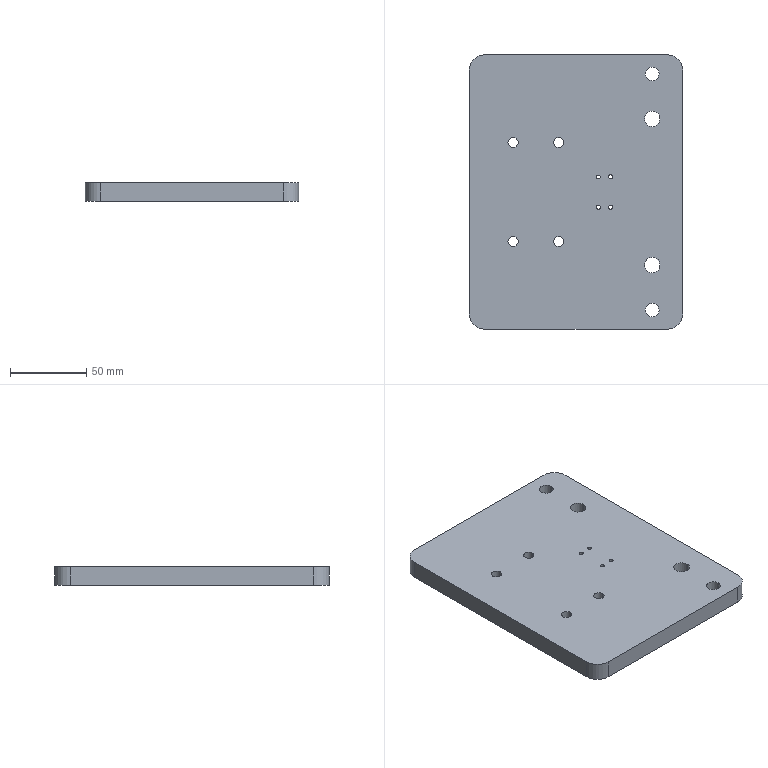Part | STEP file | Base plate 1_Default<Machined> | 1 solid | 34 faces | box 140 x 180 x 12 mm | volume 295903 mm3 | cylinder 28 | plane 6 | commonest cylinder face diameters 2.5 x8 6.8 x8 9 x4 10.2 x4 20 x4
STEP:
#1=CARTESIAN_POINT('',(21.45,-10.,0.));
#2=VERTEX_POINT('',#1);
#3=CARTESIAN_POINT('',(23.95,-10.,0.));
#4=VERTEX_POINT('',#3);
#5=CARTESIAN_POINT('',(22.7,-10.,0.));
#6=DIRECTION('',(0.,0.,1.));
#7=DIRECTION('',(1.,0.,0.));
#8=AXIS2_PLACEMENT_3D('',#5,#6,#7);
#9=CIRCLE('',#8,1.25);
#10=EDGE_CURVE('',#2,#4,#9,.T.);
#11=ORIENTED_EDGE('',*,*,#10,.F.);
#12=CARTESIAN_POINT('',(21.45,-10.,12.));
#13=VERTEX_POINT('',#12);
#14=CARTESIAN_POINT('',(21.45,-10.,12.));
#15=DIRECTION('',(0.,0.,1.));
#16=VECTOR('',#15,1000.);
#17=LINE('',#14,#16);
#18=EDGE_CURVE('',#2,#13,#17,.T.);
#19=ORIENTED_EDGE('',*,*,#18,.T.);
#20=CARTESIAN_POINT('',(23.95,-10.,12.));
#21=VERTEX_POINT('',#20);
#22=CARTESIAN_POINT('',(22.7,-10.,12.));
#23=DIRECTION('',(0.,0.,1.));
#24=DIRECTION('',(1.,0.,0.));
#25=AXIS2_PLACEMENT_3D('',#22,#23,#24);
#26=CIRCLE('',#25,1.25);
#27=EDGE_CURVE('',#13,#21,#26,.T.);
#28=ORIENTED_EDGE('',*,*,#27,.T.);
#29=CARTESIAN_POINT('',(23.95,-10.,12.));
#30=DIRECTION('',(0.,0.,1.));
#31=VECTOR('',#30,1000.);
#32=LINE('',#29,#31);
#33=EDGE_CURVE('',#4,#21,#32,.T.);
#34=ORIENTED_EDGE('',*,*,#33,.F.);
#35=EDGE_LOOP('',(#11,#19,#28,#34));
#36=FACE_OUTER_BOUND('',#35,.T.);
#37=CARTESIAN_POINT('',(22.7,-10.,12.));
#38=DIRECTION('',(0.,0.,1.));
#39=DIRECTION('',(1.,0.,0.));
#40=AXIS2_PLACEMENT_3D('',#37,#38,#39);
#41=CYLINDRICAL_SURFACE('',#40,1.25);
#42=ADVANCED_FACE('',(#36),#41,.F.);
#43=CARTESIAN_POINT('',(13.45,-10.,0.));
#44=VERTEX_POINT('',#43);
#45=CARTESIAN_POINT('',(15.95,-10.,0.));
#46=VERTEX_POINT('',#45);
#47=CARTESIAN_POINT('',(14.7,-10.,0.));
#48=DIRECTION('',(0.,0.,1.));
#49=DIRECTION('',(1.,0.,0.));
#50=AXIS2_PLACEMENT_3D('',#47,#48,#49);
#51=CIRCLE('',#50,1.25);
#52=EDGE_CURVE('',#44,#46,#51,.T.);
#53=ORIENTED_EDGE('',*,*,#52,.F.);
#54=CARTESIAN_POINT('',(13.45,-10.,12.));
#55=VERTEX_POINT('',#54);
#56=CARTESIAN_POINT('',(13.45,-10.,12.));
#57=DIRECTION('',(0.,0.,1.));
#58=VECTOR('',#57,1000.);
#59=LINE('',#56,#58);
#60=EDGE_CURVE('',#44,#55,#59,.T.);
#61=ORIENTED_EDGE('',*,*,#60,.T.);
#62=CARTESIAN_POINT('',(15.95,-10.,12.));
#63=VERTEX_POINT('',#62);
#64=CARTESIAN_POINT('',(14.7,-10.,12.));
#65=DIRECTION('',(0.,0.,1.));
#66=DIRECTION('',(1.,0.,0.));
#67=AXIS2_PLACEMENT_3D('',#64,#65,#66);
#68=CIRCLE('',#67,1.25);
#69=EDGE_CURVE('',#55,#63,#68,.T.);
#70=ORIENTED_EDGE('',*,*,#69,.T.);
#71=CARTESIAN_POINT('',(15.95,-10.,12.));
#72=DIRECTION('',(0.,0.,1.));
#73=VECTOR('',#72,1000.);
#74=LINE('',#71,#73);
#75=EDGE_CURVE('',#46,#63,#74,.T.);
#76=ORIENTED_EDGE('',*,*,#75,.F.);
#77=EDGE_LOOP('',(#53,#61,#70,#76));
#78=FACE_OUTER_BOUND('',#77,.T.);
#79=CARTESIAN_POINT('',(14.7,-10.,12.));
#80=DIRECTION('',(0.,0.,1.));
#81=DIRECTION('',(1.,0.,0.));
#82=AXIS2_PLACEMENT_3D('',#79,#80,#81);
#83=CYLINDRICAL_SURFACE('',#82,1.25);
#84=ADVANCED_FACE('',(#78),#83,.F.);
#85=CARTESIAN_POINT('',(21.45,10.,0.));
#86=VERTEX_POINT('',#85);
#87=CARTESIAN_POINT('',(23.95,10.,0.));
#88=VERTEX_POINT('',#87);
#89=CARTESIAN_POINT('',(22.7,10.,0.));
#90=DIRECTION('',(0.,0.,1.));
#91=DIRECTION('',(1.,0.,0.));
#92=AXIS2_PLACEMENT_3D('',#89,#90,#91);
#93=CIRCLE('',#92,1.25);
#94=EDGE_CURVE('',#86,#88,#93,.T.);
#95=ORIENTED_EDGE('',*,*,#94,.F.);
#96=CARTESIAN_POINT('',(21.45,10.,12.));
#97=VERTEX_POINT('',#96);
#98=CARTESIAN_POINT('',(21.45,10.,12.));
#99=DIRECTION('',(0.,0.,1.));
#100=VECTOR('',#99,1000.);
#101=LINE('',#98,#100);
#102=EDGE_CURVE('',#86,#97,#101,.T.);
#103=ORIENTED_EDGE('',*,*,#102,.T.);
#104=CARTESIAN_POINT('',(23.95,10.,12.));
#105=VERTEX_POINT('',#104);
#106=CARTESIAN_POINT('',(22.7,10.,12.));
#107=DIRECTION('',(0.,0.,1.));
#108=DIRECTION('',(1.,0.,0.));
#109=AXIS2_PLACEMENT_3D('',#106,#107,#108);
#110=CIRCLE('',#109,1.25);
#111=EDGE_CURVE('',#97,#105,#110,.T.);
#112=ORIENTED_EDGE('',*,*,#111,.T.);
#113=CARTESIAN_POINT('',(23.95,10.,12.));
#114=DIRECTION('',(0.,0.,1.));
#115=VECTOR('',#114,1000.);
#116=LINE('',#113,#115);
#117=EDGE_CURVE('',#88,#105,#116,.T.);
#118=ORIENTED_EDGE('',*,*,#117,.F.);
#119=EDGE_LOOP('',(#95,#103,#112,#118));
#120=FACE_OUTER_BOUND('',#119,.T.);
#121=CARTESIAN_POINT('',(22.7,10.,12.));
#122=DIRECTION('',(0.,0.,1.));
#123=DIRECTION('',(1.,0.,0.));
#124=AXIS2_PLACEMENT_3D('',#121,#122,#123);
#125=CYLINDRICAL_SURFACE('',#124,1.25);
#126=ADVANCED_FACE('',(#120),#125,.F.);
#127=CARTESIAN_POINT('',(13.45,9.85,0.));
#128=VERTEX_POINT('',#127);
#129=CARTESIAN_POINT('',(15.95,9.85,0.));
#130=VERTEX_POINT('',#129);
#131=CARTESIAN_POINT('',(14.7,9.85,0.));
#132=DIRECTION('',(0.,0.,1.));
#133=DIRECTION('',(1.,0.,0.));
#134=AXIS2_PLACEMENT_3D('',#131,#132,#133);
#135=CIRCLE('',#134,1.25);
#136=EDGE_CURVE('',#128,#130,#135,.T.);
#137=ORIENTED_EDGE('',*,*,#136,.F.);
#138=CARTESIAN_POINT('',(13.45,9.85,12.));
#139=VERTEX_POINT('',#138);
#140=CARTESIAN_POINT('',(13.45,9.85,12.));
#141=DIRECTION('',(0.,0.,1.));
#142=VECTOR('',#141,1000.);
#143=LINE('',#140,#142);
#144=EDGE_CURVE('',#128,#139,#143,.T.);
#145=ORIENTED_EDGE('',*,*,#144,.T.);
#146=CARTESIAN_POINT('',(15.95,9.85,12.));
#147=VERTEX_POINT('',#146);
#148=CARTESIAN_POINT('',(14.7,9.85,12.));
#149=DIRECTION('',(0.,0.,1.));
#150=DIRECTION('',(1.,0.,0.));
#151=AXIS2_PLACEMENT_3D('',#148,#149,#150);
#152=CIRCLE('',#151,1.25);
#153=EDGE_CURVE('',#139,#147,#152,.T.);
#154=ORIENTED_EDGE('',*,*,#153,.T.);
#155=CARTESIAN_POINT('',(15.95,9.85,12.));
#156=DIRECTION('',(0.,0.,1.));
#157=VECTOR('',#156,1000.);
#158=LINE('',#155,#157);
#159=EDGE_CURVE('',#130,#147,#158,.T.);
#160=ORIENTED_EDGE('',*,*,#159,.F.);
#161=EDGE_LOOP('',(#137,#145,#154,#160));
#162=FACE_OUTER_BOUND('',#161,.T.);
#163=CARTESIAN_POINT('',(14.7,9.85,12.));
#164=DIRECTION('',(0.,0.,1.));
#165=DIRECTION('',(1.,0.,0.));
#166=AXIS2_PLACEMENT_3D('',#163,#164,#165);
#167=CYLINDRICAL_SURFACE('',#166,1.25);
#168=ADVANCED_FACE('',(#162),#167,.F.);
#169=CARTESIAN_POINT('',(45.5,77.5,0.));
#170=VERTEX_POINT('',#169);
#171=CARTESIAN_POINT('',(54.5,77.5,0.));
#172=VERTEX_POINT('',#171);
#173=CARTESIAN_POINT('',(50.,77.5,0.));
#174=DIRECTION('',(0.,0.,1.));
#175=DIRECTION('',(1.,0.,0.));
#176=AXIS2_PLACEMENT_3D('',#173,#174,#175);
#177=CIRCLE('',#176,4.5);
#178=EDGE_CURVE('',#170,#172,#177,.T.);
#179=ORIENTED_EDGE('',*,*,#178,.F.);
#180=CARTESIAN_POINT('',(45.5,77.5,12.));
#181=VERTEX_POINT('',#180);
#182=CARTESIAN_POINT('',(45.5,77.5,12.));
#183=DIRECTION('',(0.,0.,1.));
#184=VECTOR('',#183,1000.);
#185=LINE('',#182,#184);
#186=EDGE_CURVE('',#170,#181,#185,.T.);
#187=ORIENTED_EDGE('',*,*,#186,.T.);
#188=CARTESIAN_POINT('',(54.5,77.5,12.));
#189=VERTEX_POINT('',#188);
#190=CARTESIAN_POINT('',(50.,77.5,12.));
#191=DIRECTION('',(0.,0.,1.));
#192=DIRECTION('',(1.,0.,0.));
#193=AXIS2_PLACEMENT_3D('',#190,#191,#192);
#194=CIRCLE('',#193,4.5);
#195=EDGE_CURVE('',#181,#189,#194,.T.);
#196=ORIENTED_EDGE('',*,*,#195,.T.);
#197=CARTESIAN_POINT('',(54.5,77.5,12.));
#198=DIRECTION('',(0.,0.,1.));
#199=VECTOR('',#198,1000.);
#200=LINE('',#197,#199);
#201=EDGE_CURVE('',#172,#189,#200,.T.);
#202=ORIENTED_EDGE('',*,*,#201,.F.);
#203=EDGE_LOOP('',(#179,#187,#196,#202));
#204=FACE_OUTER_BOUND('',#203,.T.);
#205=CARTESIAN_POINT('',(50.,77.5,12.));
#206=DIRECTION('',(0.,0.,1.));
#207=DIRECTION('',(1.,0.,0.));
#208=AXIS2_PLACEMENT_3D('',#205,#206,#207);
#209=CYLINDRICAL_SURFACE('',#208,4.5);
#210=ADVANCED_FACE('',(#204),#209,.F.);
#211=CARTESIAN_POINT('',(45.5,-77.5,0.));
#212=VERTEX_POINT('',#211);
#213=CARTESIAN_POINT('',(54.5,-77.5,0.));
#214=VERTEX_POINT('',#213);
#215=CARTESIAN_POINT('',(50.,-77.5,0.));
#216=DIRECTION('',(0.,0.,1.));
#217=DIRECTION('',(1.,0.,0.));
#218=AXIS2_PLACEMENT_3D('',#215,#216,#217);
#219=CIRCLE('',#218,4.5);
#220=EDGE_CURVE('',#212,#214,#219,.T.);
#221=ORIENTED_EDGE('',*,*,#220,.F.);
#222=CARTESIAN_POINT('',(45.5,-77.5,12.));
#223=VERTEX_POINT('',#222);
#224=CARTESIAN_POINT('',(45.5,-77.5,12.));
#225=DIRECTION('',(0.,0.,1.));
#226=VECTOR('',#225,1000.);
#227=LINE('',#224,#226);
#228=EDGE_CURVE('',#212,#223,#227,.T.);
#229=ORIENTED_EDGE('',*,*,#228,.T.);
#230=CARTESIAN_POINT('',(54.5,-77.5,12.));
#231=VERTEX_POINT('',#230);
#232=CARTESIAN_POINT('',(50.,-77.5,12.));
#233=DIRECTION('',(0.,0.,1.));
#234=DIRECTION('',(1.,0.,0.));
#235=AXIS2_PLACEMENT_3D('',#232,#233,#234);
#236=CIRCLE('',#235,4.5);
#237=EDGE_CURVE('',#223,#231,#236,.T.);
#238=ORIENTED_EDGE('',*,*,#237,.T.);
#239=CARTESIAN_POINT('',(54.5,-77.5,12.));
#240=DIRECTION('',(0.,0.,1.));
#241=VECTOR('',#240,1000.);
#242=LINE('',#239,#241);
#243=EDGE_CURVE('',#214,#231,#242,.T.);
#244=ORIENTED_EDGE('',*,*,#243,.F.);
#245=EDGE_LOOP('',(#221,#229,#238,#244));
#246=FACE_OUTER_BOUND('',#245,.T.);
#247=CARTESIAN_POINT('',(50.,-77.5,12.));
#248=DIRECTION('',(0.,0.,1.));
#249=DIRECTION('',(1.,0.,0.));
#250=AXIS2_PLACEMENT_3D('',#247,#248,#249);
#251=CYLINDRICAL_SURFACE('',#250,4.5);
#252=ADVANCED_FACE('',(#246),#251,.F.);
#253=CARTESIAN_POINT('',(44.9,48.,0.));
#254=VERTEX_POINT('',#253);
#255=CARTESIAN_POINT('',(55.1,48.,0.));
#256=VERTEX_POINT('',#255);
#257=CARTESIAN_POINT('',(50.,48.,0.));
#258=DIRECTION('',(0.,0.,1.));
#259=DIRECTION('',(1.,0.,0.));
#260=AXIS2_PLACEMENT_3D('',#257,#258,#259);
#261=CIRCLE('',#260,5.1);
#262=EDGE_CURVE('',#254,#256,#261,.T.);
#263=ORIENTED_EDGE('',*,*,#262,.F.);
#264=CARTESIAN_POINT('',(44.9,48.,12.));
#265=VERTEX_POINT('',#264);
#266=CARTESIAN_POINT('',(44.9,48.,12.));
#267=DIRECTION('',(0.,0.,1.));
#268=VECTOR('',#267,1000.);
#269=LINE('',#266,#268);
#270=EDGE_CURVE('',#254,#265,#269,.T.);
#271=ORIENTED_EDGE('',*,*,#270,.T.);
#272=CARTESIAN_POINT('',(55.1,48.,12.));
#273=VERTEX_POINT('',#272);
#274=CARTESIAN_POINT('',(50.,48.,12.));
#275=DIRECTION('',(0.,0.,1.));
#276=DIRECTION('',(1.,0.,0.));
#277=AXIS2_PLACEMENT_3D('',#274,#275,#276);
#278=CIRCLE('',#277,5.1);
#279=EDGE_CURVE('',#265,#273,#278,.T.);
#280=ORIENTED_EDGE('',*,*,#279,.T.);
#281=CARTESIAN_POINT('',(55.1,48.,12.));
#282=DIRECTION('',(0.,0.,1.));
#283=VECTOR('',#282,1000.);
#284=LINE('',#281,#283);
#285=EDGE_CURVE('',#256,#273,#284,.T.);
#286=ORIENTED_EDGE('',*,*,#285,.F.);
#287=EDGE_LOOP('',(#263,#271,#280,#286));
#288=FACE_OUTER_BOUND('',#287,.T.);
#289=CARTESIAN_POINT('',(50.,48.,12.));
#290=DIRECTION('',(0.,0.,1.));
#291=DIRECTION('',(1.,0.,0.));
#292=AXIS2_PLACEMENT_3D('',#289,#290,#291);
#293=CYLINDRICAL_SURFACE('',#292,5.1);
#294=ADVANCED_FACE('',(#288),#293,.F.);
#295=CARTESIAN_POINT('',(44.9,-48.,0.));
#296=VERTEX_POINT('',#295);
#297=CARTESIAN_POINT('',(55.1,-48.,0.));
#298=VERTEX_POINT('',#297);
#299=CARTESIAN_POINT('',(50.,-48.,0.));
#300=DIRECTION('',(0.,0.,1.));
#301=DIRECTION('',(1.,0.,0.));
#302=AXIS2_PLACEMENT_3D('',#299,#300,#301);
#303=CIRCLE('',#302,5.1);
#304=EDGE_CURVE('',#296,#298,#303,.T.);
#305=ORIENTED_EDGE('',*,*,#304,.F.);
#306=CARTESIAN_POINT('',(44.9,-48.,12.));
#307=VERTEX_POINT('',#306);
#308=CARTESIAN_POINT('',(44.9,-48.,12.));
#309=DIRECTION('',(0.,0.,1.));
#310=VECTOR('',#309,1000.);
#311=LINE('',#308,#310);
#312=EDGE_CURVE('',#296,#307,#311,.T.);
#313=ORIENTED_EDGE('',*,*,#312,.T.);
#314=CARTESIAN_POINT('',(55.1,-48.,12.));
#315=VERTEX_POINT('',#314);
#316=CARTESIAN_POINT('',(50.,-48.,12.));
#317=DIRECTION('',(0.,0.,1.));
#318=DIRECTION('',(1.,0.,0.));
#319=AXIS2_PLACEMENT_3D('',#316,#317,#318);
#320=CIRCLE('',#319,5.1);
#321=EDGE_CURVE('',#307,#315,#320,.T.);
#322=ORIENTED_EDGE('',*,*,#321,.T.);
#323=CARTESIAN_POINT('',(55.1,-48.,12.));
#324=DIRECTION('',(0.,0.,1.));
#325=VECTOR('',#324,1000.);
#326=LINE('',#323,#325);
#327=EDGE_CURVE('',#298,#315,#326,.T.);
#328=ORIENTED_EDGE('',*,*,#327,.F.);
#329=EDGE_LOOP('',(#305,#313,#322,#328));
#330=FACE_OUTER_BOUND('',#329,.T.);
#331=CARTESIAN_POINT('',(50.,-48.,12.));
#332=DIRECTION('',(0.,0.,1.));
#333=DIRECTION('',(1.,0.,0.));
#334=AXIS2_PLACEMENT_3D('',#331,#332,#333);
#335=CYLINDRICAL_SURFACE('',#334,5.1);
#336=ADVANCED_FACE('',(#330),#335,.F.);
#337=CARTESIAN_POINT('',(-14.7,32.5,0.));
#338=VERTEX_POINT('',#337);
#339=CARTESIAN_POINT('',(-7.9,32.5,0.));
#340=VERTEX_POINT('',#339);
#341=CARTESIAN_POINT('',(-11.3,32.5,0.));
#342=DIRECTION('',(0.,0.,1.));
#343=DIRECTION('',(1.,0.,0.));
#344=AXIS2_PLACEMENT_3D('',#341,#342,#343);
#345=CIRCLE('',#344,3.4);
#346=EDGE_CURVE('',#338,#340,#345,.T.);
#347=ORIENTED_EDGE('',*,*,#346,.F.);
#348=CARTESIAN_POINT('',(-14.7,32.5,12.));
#349=VERTEX_POINT('',#348);
#350=CARTESIAN_POINT('',(-14.7,32.5,12.));
#351=DIRECTION('',(0.,0.,1.));
#352=VECTOR('',#351,1000.);
#353=LINE('',#350,#352);
#354=EDGE_CURVE('',#338,#349,#353,.T.);
#355=ORIENTED_EDGE('',*,*,#354,.T.);
#356=CARTESIAN_POINT('',(-7.9,32.5,12.));
#357=VERTEX_POINT('',#356);
#358=CARTESIAN_POINT('',(-11.3,32.5,12.));
#359=DIRECTION('',(0.,0.,1.));
#360=DIRECTION('',(1.,0.,0.));
#361=AXIS2_PLACEMENT_3D('',#358,#359,#360);
#362=CIRCLE('',#361,3.4);
#363=EDGE_CURVE('',#349,#357,#362,.T.);
#364=ORIENTED_EDGE('',*,*,#363,.T.);
#365=CARTESIAN_POINT('',(-7.9,32.5,12.));
#366=DIRECTION('',(0.,0.,1.));
#367=VECTOR('',#366,1000.);
#368=LINE('',#365,#367);
#369=EDGE_CURVE('',#340,#357,#368,.T.);
#370=ORIENTED_EDGE('',*,*,#369,.F.);
#371=EDGE_LOOP('',(#347,#355,#364,#370));
#372=FACE_OUTER_BOUND('',#371,.T.);
#373=CARTESIAN_POINT('',(-11.3,32.5,12.));
#374=DIRECTION('',(0.,0.,1.));
#375=DIRECTION('',(1.,0.,0.));
#376=AXIS2_PLACEMENT_3D('',#373,#374,#375);
#377=CYLINDRICAL_SURFACE('',#376,3.4);
#378=ADVANCED_FACE('',(#372),#377,.F.);
#379=CARTESIAN_POINT('',(-44.7,32.5,0.));
#380=VERTEX_POINT('',#379);
#381=CARTESIAN_POINT('',(-37.9,32.5,0.));
#382=VERTEX_POINT('',#381);
#383=CARTESIAN_POINT('',(-41.3,32.5,0.));
#384=DIRECTION('',(0.,0.,1.));
#385=DIRECTION('',(1.,0.,0.));
#386=AXIS2_PLACEMENT_3D('',#383,#384,#385);
#387=CIRCLE('',#386,3.4);
#388=EDGE_CURVE('',#380,#382,#387,.T.);
#389=ORIENTED_EDGE('',*,*,#388,.F.);
#390=CARTESIAN_POINT('',(-44.7,32.5,12.));
#391=VERTEX_POINT('',#390);
#392=CARTESIAN_POINT('',(-44.7,32.5,12.));
#393=DIRECTION('',(0.,0.,1.));
#394=VECTOR('',#393,1000.);
#395=LINE('',#392,#394);
#396=EDGE_CURVE('',#380,#391,#395,.T.);
#397=ORIENTED_EDGE('',*,*,#396,.T.);
#398=CARTESIAN_POINT('',(-37.9,32.5,12.));
#399=VERTEX_POINT('',#398);
#400=CARTESIAN_POINT('',(-41.3,32.5,12.));
#401=DIRECTION('',(0.,0.,1.));
#402=DIRECTION('',(1.,0.,0.));
#403=AXIS2_PLACEMENT_3D('',#400,#401,#402);
#404=CIRCLE('',#403,3.4);
#405=EDGE_CURVE('',#391,#399,#404,.T.);
#406=ORIENTED_EDGE('',*,*,#405,.T.);
#407=CARTESIAN_POINT('',(-37.9,32.5,12.));
#408=DIRECTION('',(0.,0.,1.));
#409=VECTOR('',#408,1000.);
#410=LINE('',#407,#409);
#411=EDGE_CURVE('',#382,#399,#410,.T.);
#412=ORIENTED_EDGE('',*,*,#411,.F.);
#413=EDGE_LOOP('',(#389,#397,#406,#412));
#414=FACE_OUTER_BOUND('',#413,.T.);
#415=CARTESIAN_POINT('',(-41.3,32.5,12.));
#416=DIRECTION('',(0.,0.,1.));
#417=DIRECTION('',(1.,0.,0.));
#418=AXIS2_PLACEMENT_3D('',#415,#416,#417);
#419=CYLINDRICAL_SURFACE('',#418,3.4);
#420=ADVANCED_FACE('',(#414),#419,.F.);
#421=CARTESIAN_POINT('',(-14.7,-32.5,0.));
#422=VERTEX_POINT('',#421);
#423=CARTESIAN_POINT('',(-7.9,-32.5,0.));
#424=VERTEX_POINT('',#423);
#425=CARTESIAN_POINT('',(-11.3,-32.5,0.));
#426=DIRECTION('',(0.,0.,1.));
#427=DIRECTION('',(1.,0.,0.));
#428=AXIS2_PLACEMENT_3D('',#425,#426,#427);
#429=CIRCLE('',#428,3.4);
#430=EDGE_CURVE('',#422,#424,#429,.T.);
#431=ORIENTED_EDGE('',*,*,#430,.F.);
#432=CARTESIAN_POINT('',(-14.7,-32.5,12.));
#433=VERTEX_POINT('',#432);
#434=CARTESIAN_POINT('',(-14.7,-32.5,12.));
#435=DIRECTION('',(0.,0.,1.));
#436=VECTOR('',#435,1000.);
#437=LINE('',#434,#436);
#438=EDGE_CURVE('',#422,#433,#437,.T.);
#439=ORIENTED_EDGE('',*,*,#438,.T.);
#440=CARTESIAN_POINT('',(-7.9,-32.5,12.));
#441=VERTEX_POINT('',#440);
#442=CARTESIAN_POINT('',(-11.3,-32.5,12.));
#443=DIRECTION('',(0.,0.,1.));
#444=DIRECTION('',(1.,0.,0.));
#445=AXIS2_PLACEMENT_3D('',#442,#443,#444);
#446=CIRCLE('',#445,3.4);
#447=EDGE_CURVE('',#433,#441,#446,.T.);
#448=ORIENTED_EDGE('',*,*,#447,.T.);
#449=CARTESIAN_POINT('',(-7.9,-32.5,12.));
#450=DIRECTION('',(0.,0.,1.));
#451=VECTOR('',#450,1000.);
#452=LINE('',#449,#451);
#453=EDGE_CURVE('',#424,#441,#452,.T.);
#454=ORIENTED_EDGE('',*,*,#453,.F.);
#455=EDGE_LOOP('',(#431,#439,#448,#454));
#456=FACE_OUTER_BOUND('',#455,.T.);
#457=CARTESIAN_POINT('',(-11.3,-32.5,12.));
#458=DIRECTION('',(0.,0.,1.));
#459=DIRECTION('',(1.,0.,0.));
#460=AXIS2_PLACEMENT_3D('',#457,#458,#459);
#461=CYLINDRICAL_SURFACE('',#460,3.4);
#462=ADVANCED_FACE('',(#456),#461,.F.);
#463=CARTESIAN_POINT('',(-44.7,-32.5,0.));
#464=VERTEX_POINT('',#463);
#465=CARTESIAN_POINT('',(-37.9,-32.5,0.));
#466=VERTEX_POINT('',#465);
#467=CARTESIAN_POINT('',(-41.3,-32.5,0.));
#468=DIRECTION('',(0.,0.,1.));
#469=DIRECTION('',(1.,0.,0.));
#470=AXIS2_PLACEMENT_3D('',#467,#468,#469);
#471=CIRCLE('',#470,3.4);
#472=EDGE_CURVE('',#464,#466,#471,.T.);
#473=ORIENTED_EDGE('',*,*,#472,.F.);
#474=CARTESIAN_POINT('',(-44.7,-32.5,12.));
#475=VERTEX_POINT('',#474);
#476=CARTESIAN_POINT('',(-44.7,-32.5,12.));
#477=DIRECTION('',(0.,0.,1.));
#478=VECTOR('',#477,1000.);
#479=LINE('',#476,#478);
#480=EDGE_CURVE('',#464,#475,#479,.T.);
#481=ORIENTED_EDGE('',*,*,#480,.T.);
#482=CARTESIAN_POINT('',(-37.9,-32.5,12.));
#483=VERTEX_POINT('',#482);
#484=CARTESIAN_POINT('',(-41.3,-32.5,12.));
#485=DIRECTION('',(0.,0.,1.));
#486=DIRECTION('',(1.,0.,0.));
#487=AXIS2_PLACEMENT_3D('',#484,#485,#486);
#488=CIRCLE('',#487,3.4);
#489=EDGE_CURVE('',#475,#483,#488,.T.);
#490=ORIENTED_EDGE('',*,*,#489,.T.);
#491=CARTESIAN_POINT('',(-37.9,-32.5,12.));
#492=DIRECTION('',(0.,0.,1.));
#493=VECTOR('',#492,1000.);
#494=LINE('',#491,#493);
#495=EDGE_CURVE('',#466,#483,#494,.T.);
#496=ORIENTED_EDGE('',*,*,#495,.F.);
#497=EDGE_LOOP('',(#473,#481,#490,#496));
#498=FACE_OUTER_BOUND('',#497,.T.);
#499=CARTESIAN_POINT('',(-41.3,-32.5,12.));
#500=DIRECTION('',(0.,0.,1.));
#501=DIRECTION('',(1.,0.,0.));
#502=AXIS2_PLACEMENT_3D('',#499,#500,#501);
#503=CYLINDRICAL_SURFACE('',#502,3.4);
#504=ADVANCED_FACE('',(#498),#503,.F.);
#505=CARTESIAN_POINT('',(70.,-80.,12.));
#506=VERTEX_POINT('',#505);
#507=CARTESIAN_POINT('',(70.,80.,12.));
#508=VERTEX_POINT('',#507);
#509=CARTESIAN_POINT('',(70.,90.,12.));
#510=DIRECTION('',(0.,1.,0.));
#511=VECTOR('',#510,1000.);
#512=LINE('',#509,#511);
#513=EDGE_CURVE('',#506,#508,#512,.T.);
#514=ORIENTED_EDGE('',*,*,#513,.F.);
#515=CARTESIAN_POINT('',(70.,-80.,0.));
#516=VERTEX_POINT('',#515);
#517=CARTESIAN_POINT('',(70.,-80.,12.));
#518=DIRECTION('',(0.,0.,-1.));
#519=VECTOR('',#518,1000.);
#520=LINE('',#517,#519);
#521=EDGE_CURVE('',#506,#516,#520,.T.);
#522=ORIENTED_EDGE('',*,*,#521,.T.);
#523=CARTESIAN_POINT('',(70.,80.,0.));
#524=VERTEX_POINT('',#523);
#525=CARTESIAN_POINT('',(70.,90.,0.));
#526=DIRECTION('',(0.,1.,0.));
#527=VECTOR('',#526,1000.);
#528=LINE('',#525,#527);
#529=EDGE_CURVE('',#516,#524,#528,.T.);
#530=ORIENTED_EDGE('',*,*,#529,.T.);
#531=CARTESIAN_POINT('',(70.,80.,12.));
#532=DIRECTION('',(0.,0.,1.));
#533=VECTOR('',#532,1000.);
#534=LINE('',#531,#533);
#535=EDGE_CURVE('',#524,#508,#534,.T.);
#536=ORIENTED_EDGE('',*,*,#535,.T.);
#537=EDGE_LOOP('',(#514,#522,#530,#536));
#538=FACE_OUTER_BOUND('',#537,.T.);
#539=CARTESIAN_POINT('',(70.,90.,12.));
#540=DIRECTION('',(-1.,0.,0.));
#541=DIRECTION('',(0.,-1.,0.));
#542=AXIS2_PLACEMENT_3D('',#539,#540,#541);
#543=PLANE('',#542);
#544=ADVANCED_FACE('',(#538),#543,.F.);
#545=CARTESIAN_POINT('',(60.,90.,12.));
#546=VERTEX_POINT('',#545);
#547=CARTESIAN_POINT('',(-60.,90.,12.));
#548=VERTEX_POINT('',#547);
#549=CARTESIAN_POINT('',(-70.,90.,12.));
#550=DIRECTION('',(-1.,0.,0.));
#551=VECTOR('',#550,1000.);
#552=LINE('',#549,#551);
#553=EDGE_CURVE('',#546,#548,#552,.T.);
#554=ORIENTED_EDGE('',*,*,#553,.F.);
#555=CARTESIAN_POINT('',(60.,90.,0.));
#556=VERTEX_POINT('',#555);
#557=CARTESIAN_POINT('',(60.,90.,12.));
#558=DIRECTION('',(0.,0.,-1.));
#559=VECTOR('',#558,1000.);
#560=LINE('',#557,#559);
#561=EDGE_CURVE('',#546,#556,#560,.T.);
#562=ORIENTED_EDGE('',*,*,#561,.T.);
#563=CARTESIAN_POINT('',(-60.,90.,0.));
#564=VERTEX_POINT('',#563);
#565=CARTESIAN_POINT('',(-70.,90.,0.));
#566=DIRECTION('',(-1.,0.,0.));
#567=VECTOR('',#566,1000.);
#568=LINE('',#565,#567);
#569=EDGE_CURVE('',#556,#564,#568,.T.);
#570=ORIENTED_EDGE('',*,*,#569,.T.);
#571=CARTESIAN_POINT('',(-60.,90.,12.));
#572=DIRECTION('',(0.,0.,1.));
#573=VECTOR('',#572,1000.);
#574=LINE('',#571,#573);
#575=EDGE_CURVE('',#564,#548,#574,.T.);
#576=ORIENTED_EDGE('',*,*,#575,.T.);
#577=EDGE_LOOP('',(#554,#562,#570,#576));
#578=FACE_OUTER_BOUND('',#577,.T.);
#579=CARTESIAN_POINT('',(-70.,90.,12.));
#580=DIRECTION('',(0.,-1.,0.));
#581=DIRECTION('',(0.,0.,-1.));
#582=AXIS2_PLACEMENT_3D('',#579,#580,#581);
#583=PLANE('',#582);
#584=ADVANCED_FACE('',(#578),#583,.F.);
#585=CARTESIAN_POINT('',(-70.,80.,0.));
#586=VERTEX_POINT('',#585);
#587=CARTESIAN_POINT('',(-70.,-80.,0.));
#588=VERTEX_POINT('',#587);
#589=CARTESIAN_POINT('',(-70.,90.,0.));
#590=DIRECTION('',(0.,-1.,0.));
#591=VECTOR('',#590,1000.);
#592=LINE('',#589,#591);
#593=EDGE_CURVE('',#586,#588,#592,.T.);
#594=ORIENTED_EDGE('',*,*,#593,.T.);
#595=CARTESIAN_POINT('',(-70.,-80.,12.));
#596=VERTEX_POINT('',#595);
#597=CARTESIAN_POINT('',(-70.,-80.,12.));
#598=DIRECTION('',(0.,0.,1.));
#599=VECTOR('',#598,1000.);
#600=LINE('',#597,#599);
#601=EDGE_CURVE('',#588,#596,#600,.T.);
#602=ORIENTED_EDGE('',*,*,#601,.T.);
#603=CARTESIAN_POINT('',(-70.,80.,12.));
#604=VERTEX_POINT('',#603);
#605=CARTESIAN_POINT('',(-70.,90.,12.));
#606=DIRECTION('',(0.,-1.,0.));
#607=VECTOR('',#606,1000.);
#608=LINE('',#605,#607);
#609=EDGE_CURVE('',#604,#596,#608,.T.);
#610=ORIENTED_EDGE('',*,*,#609,.F.);
#611=CARTESIAN_POINT('',(-70.,80.,12.));
#612=DIRECTION('',(0.,0.,-1.));
#613=VECTOR('',#612,1000.);
#614=LINE('',#611,#613);
#615=EDGE_CURVE('',#604,#586,#614,.T.);
#616=ORIENTED_EDGE('',*,*,#615,.T.);
#617=EDGE_LOOP('',(#594,#602,#610,#616));
#618=FACE_OUTER_BOUND('',#617,.T.);
#619=CARTESIAN_POINT('',(-70.,90.,12.));
#620=DIRECTION('',(1.,0.,0.));
#621=DIRECTION('',(0.,1.,0.));
#622=AXIS2_PLACEMENT_3D('',#619,#620,#621);
#623=PLANE('',#622);
#624=ADVANCED_FACE('',(#618),#623,.F.);
#625=CARTESIAN_POINT('',(-60.,-90.,12.));
#626=VERTEX_POINT('',#625);
#627=CARTESIAN_POINT('',(60.,-90.,12.));
#628=VERTEX_POINT('',#627);
#629=CARTESIAN_POINT('',(-70.,-90.,12.));
#630=DIRECTION('',(1.,0.,0.));
#631=VECTOR('',#630,1000.);
#632=LINE('',#629,#631);
#633=EDGE_CURVE('',#626,#628,#632,.T.);
#634=ORIENTED_EDGE('',*,*,#633,.F.);
#635=CARTESIAN_POINT('',(-60.,-90.,0.));
#636=VERTEX_POINT('',#635);
#637=CARTESIAN_POINT('',(-60.,-90.,12.));
#638=DIRECTION('',(0.,0.,-1.));
#639=VECTOR('',#638,1000.);
#640=LINE('',#637,#639);
#641=EDGE_CURVE('',#626,#636,#640,.T.);
#642=ORIENTED_EDGE('',*,*,#641,.T.);
#643=CARTESIAN_POINT('',(60.,-90.,0.));
#644=VERTEX_POINT('',#643);
#645=CARTESIAN_POINT('',(-70.,-90.,0.));
#646=DIRECTION('',(1.,0.,0.));
#647=VECTOR('',#646,1000.);
#648=LINE('',#645,#647);
#649=EDGE_CURVE('',#636,#644,#648,.T.);
#650=ORIENTED_EDGE('',*,*,#649,.T.);
#651=CARTESIAN_POINT('',(60.,-90.,12.));
#652=DIRECTION('',(0.,0.,1.));
#653=VECTOR('',#652,1000.);
#654=LINE('',#651,#653);
#655=EDGE_CURVE('',#644,#628,#654,.T.);
#656=ORIENTED_EDGE('',*,*,#655,.T.);
#657=EDGE_LOOP('',(#634,#642,#650,#656));
#658=FACE_OUTER_BOUND('',#657,.T.);
#659=CARTESIAN_POINT('',(-70.,-90.,12.));
#660=DIRECTION('',(0.,1.,0.));
#661=DIRECTION('',(0.,0.,1.));
#662=AXIS2_PLACEMENT_3D('',#659,#660,#661);
#663=PLANE('',#662);
#664=ADVANCED_FACE('',(#658),#663,.F.);
#665=CARTESIAN_POINT('',(22.7,-10.,12.));
#666=DIRECTION('',(0.,0.,1.));
#667=DIRECTION('',(1.,0.,0.));
#668=AXIS2_PLACEMENT_3D('',#665,#666,#667);
#669=CIRCLE('',#668,1.25);
#670=EDGE_CURVE('',#21,#13,#669,.T.);
#671=ORIENTED_EDGE('',*,*,#670,.F.);
#672=ORIENTED_EDGE('',*,*,#27,.F.);
#673=EDGE_LOOP('',(#671,#672));
#674=FACE_BOUND('',#673,.T.);
#675=CARTESIAN_POINT('',(14.7,-10.,12.));
#676=DIRECTION('',(0.,0.,1.));
#677=DIRECTION('',(1.,0.,0.));
#678=AXIS2_PLACEMENT_3D('',#675,#676,#677);
#679=CIRCLE('',#678,1.25);
#680=EDGE_CURVE('',#63,#55,#679,.T.);
#681=ORIENTED_EDGE('',*,*,#680,.F.);
#682=ORIENTED_EDGE('',*,*,#69,.F.);
#683=EDGE_LOOP('',(#681,#682));
#684=FACE_BOUND('',#683,.T.);
#685=CARTESIAN_POINT('',(22.7,10.,12.));
#686=DIRECTION('',(0.,0.,1.));
#687=DIRECTION('',(1.,0.,0.));
#688=AXIS2_PLACEMENT_3D('',#685,#686,#687);
#689=CIRCLE('',#688,1.25);
#690=EDGE_CURVE('',#105,#97,#689,.T.);
#691=ORIENTED_EDGE('',*,*,#690,.F.);
#692=ORIENTED_EDGE('',*,*,#111,.F.);
#693=EDGE_LOOP('',(#691,#692));
#694=FACE_BOUND('',#693,.T.);
#695=CARTESIAN_POINT('',(14.7,9.85,12.));
#696=DIRECTION('',(0.,0.,1.));
#697=DIRECTION('',(1.,0.,0.));
#698=AXIS2_PLACEMENT_3D('',#695,#696,#697);
#699=CIRCLE('',#698,1.25);
#700=EDGE_CURVE('',#147,#139,#699,.T.);
#701=ORIENTED_EDGE('',*,*,#700,.F.);
#702=ORIENTED_EDGE('',*,*,#153,.F.);
#703=EDGE_LOOP('',(#701,#702));
#704=FACE_BOUND('',#703,.T.);
#705=CARTESIAN_POINT('',(50.,77.5,12.));
#706=DIRECTION('',(0.,0.,1.));
#707=DIRECTION('',(1.,0.,0.));
#708=AXIS2_PLACEMENT_3D('',#705,#706,#707);
#709=CIRCLE('',#708,4.5);
#710=EDGE_CURVE('',#189,#181,#709,.T.);
#711=ORIENTED_EDGE('',*,*,#710,.F.);
#712=ORIENTED_EDGE('',*,*,#195,.F.);
#713=EDGE_LOOP('',(#711,#712));
#714=FACE_BOUND('',#713,.T.);
#715=CARTESIAN_POINT('',(50.,-77.5,12.));
#716=DIRECTION('',(0.,0.,1.));
#717=DIRECTION('',(1.,0.,0.));
#718=AXIS2_PLACEMENT_3D('',#715,#716,#717);
#719=CIRCLE('',#718,4.5);
#720=EDGE_CURVE('',#231,#223,#719,.T.);
#721=ORIENTED_EDGE('',*,*,#720,.F.);
#722=ORIENTED_EDGE('',*,*,#237,.F.);
#723=EDGE_LOOP('',(#721,#722));
#724=FACE_BOUND('',#723,.T.);
#725=CARTESIAN_POINT('',(50.,48.,12.));
#726=DIRECTION('',(0.,0.,1.));
#727=DIRECTION('',(1.,0.,0.));
#728=AXIS2_PLACEMENT_3D('',#725,#726,#727);
#729=CIRCLE('',#728,5.1);
#730=EDGE_CURVE('',#273,#265,#729,.T.);
#731=ORIENTED_EDGE('',*,*,#730,.F.);
#732=ORIENTED_EDGE('',*,*,#279,.F.);
#733=EDGE_LOOP('',(#731,#732));
#734=FACE_BOUND('',#733,.T.);
#735=CARTESIAN_POINT('',(50.,-48.,12.));
#736=DIRECTION('',(0.,0.,1.));
#737=DIRECTION('',(1.,0.,0.));
#738=AXIS2_PLACEMENT_3D('',#735,#736,#737);
#739=CIRCLE('',#738,5.1);
#740=EDGE_CURVE('',#315,#307,#739,.T.);
#741=ORIENTED_EDGE('',*,*,#740,.F.);
#742=ORIENTED_EDGE('',*,*,#321,.F.);
#743=EDGE_LOOP('',(#741,#742));
#744=FACE_BOUND('',#743,.T.);
#745=CARTESIAN_POINT('',(-11.3,32.5,12.));
#746=DIRECTION('',(0.,0.,1.));
#747=DIRECTION('',(1.,0.,0.));
#748=AXIS2_PLACEMENT_3D('',#745,#746,#747);
#749=CIRCLE('',#748,3.4);
#750=EDGE_CURVE('',#357,#349,#749,.T.);
#751=ORIENTED_EDGE('',*,*,#750,.F.);
#752=ORIENTED_EDGE('',*,*,#363,.F.);
#753=EDGE_LOOP('',(#751,#752));
#754=FACE_BOUND('',#753,.T.);
#755=CARTESIAN_POINT('',(-41.3,32.5,12.));
#756=DIRECTION('',(0.,0.,1.));
#757=DIRECTION('',(1.,0.,0.));
#758=AXIS2_PLACEMENT_3D('',#755,#756,#757);
#759=CIRCLE('',#758,3.4);
#760=EDGE_CURVE('',#399,#391,#759,.T.);
#761=ORIENTED_EDGE('',*,*,#760,.F.);
#762=ORIENTED_EDGE('',*,*,#405,.F.);
#763=EDGE_LOOP('',(#761,#762));
#764=FACE_BOUND('',#763,.T.);
#765=CARTESIAN_POINT('',(-11.3,-32.5,12.));
#766=DIRECTION('',(0.,0.,1.));
#767=DIRECTION('',(1.,0.,0.));
#768=AXIS2_PLACEMENT_3D('',#765,#766,#767);
#769=CIRCLE('',#768,3.4);
#770=EDGE_CURVE('',#441,#433,#769,.T.);
#771=ORIENTED_EDGE('',*,*,#770,.F.);
#772=ORIENTED_EDGE('',*,*,#447,.F.);
#773=EDGE_LOOP('',(#771,#772));
#774=FACE_BOUND('',#773,.T.);
#775=CARTESIAN_POINT('',(-41.3,-32.5,12.));
#776=DIRECTION('',(0.,0.,1.));
#777=DIRECTION('',(1.,0.,0.));
#778=AXIS2_PLACEMENT_3D('',#775,#776,#777);
#779=CIRCLE('',#778,3.4);
#780=EDGE_CURVE('',#483,#475,#779,.T.);
#781=ORIENTED_EDGE('',*,*,#780,.F.);
#782=ORIENTED_EDGE('',*,*,#489,.F.);
#783=EDGE_LOOP('',(#781,#782));
#784=FACE_BOUND('',#783,.T.);
#785=ORIENTED_EDGE('',*,*,#609,.T.);
#786=CARTESIAN_POINT('',(-60.,-80.,12.));
#787=DIRECTION('',(0.,0.,1.));
#788=DIRECTION('',(1.,0.,0.));
#789=AXIS2_PLACEMENT_3D('',#786,#787,#788);
#790=CIRCLE('',#789,10.);
#791=EDGE_CURVE('',#596,#626,#790,.T.);
#792=ORIENTED_EDGE('',*,*,#791,.T.);
#793=ORIENTED_EDGE('',*,*,#633,.T.);
#794=CARTESIAN_POINT('',(60.,-80.,12.));
#795=DIRECTION('',(0.,0.,1.));
#796=DIRECTION('',(1.,0.,0.));
#797=AXIS2_PLACEMENT_3D('',#794,#795,#796);
#798=CIRCLE('',#797,10.);
#799=EDGE_CURVE('',#628,#506,#798,.T.);
#800=ORIENTED_EDGE('',*,*,#799,.T.);
#801=ORIENTED_EDGE('',*,*,#513,.T.);
#802=CARTESIAN_POINT('',(60.,80.,12.));
#803=DIRECTION('',(0.,0.,1.));
#804=DIRECTION('',(1.,0.,0.));
#805=AXIS2_PLACEMENT_3D('',#802,#803,#804);
#806=CIRCLE('',#805,10.);
#807=EDGE_CURVE('',#508,#546,#806,.T.);
#808=ORIENTED_EDGE('',*,*,#807,.T.);
#809=ORIENTED_EDGE('',*,*,#553,.T.);
#810=CARTESIAN_POINT('',(-60.,80.,12.));
#811=DIRECTION('',(0.,0.,1.));
#812=DIRECTION('',(1.,0.,0.));
#813=AXIS2_PLACEMENT_3D('',#810,#811,#812);
#814=CIRCLE('',#813,10.);
#815=EDGE_CURVE('',#548,#604,#814,.T.);
#816=ORIENTED_EDGE('',*,*,#815,.T.);
#817=EDGE_LOOP('',(#785,#792,#793,#800,#801,#808,#809,#816));
#818=FACE_OUTER_BOUND('',#817,.T.);
#819=CARTESIAN_POINT('',(0.,0.,12.));
#820=DIRECTION('',(0.,0.,1.));
#821=DIRECTION('',(1.,0.,0.));
#822=AXIS2_PLACEMENT_3D('',#819,#820,#821);
#823=PLANE('',#822);
#824=ADVANCED_FACE('',(#674,#684,#694,#704,#714,#724,#734,#744,#754,#764,#774,#784,#818),#823,.T.);
#825=CARTESIAN_POINT('',(22.7,-10.,0.));
#826=DIRECTION('',(0.,0.,1.));
#827=DIRECTION('',(1.,0.,0.));
#828=AXIS2_PLACEMENT_3D('',#825,#826,#827);
#829=CIRCLE('',#828,1.25);
#830=EDGE_CURVE('',#4,#2,#829,.T.);
#831=ORIENTED_EDGE('',*,*,#830,.T.);
#832=ORIENTED_EDGE('',*,*,#10,.T.);
#833=EDGE_LOOP('',(#831,#832));
#834=FACE_BOUND('',#833,.T.);
#835=CARTESIAN_POINT('',(14.7,-10.,0.));
#836=DIRECTION('',(0.,0.,1.));
#837=DIRECTION('',(1.,0.,0.));
#838=AXIS2_PLACEMENT_3D('',#835,#836,#837);
#839=CIRCLE('',#838,1.25);
#840=EDGE_CURVE('',#46,#44,#839,.T.);
#841=ORIENTED_EDGE('',*,*,#840,.T.);
#842=ORIENTED_EDGE('',*,*,#52,.T.);
#843=EDGE_LOOP('',(#841,#842));
#844=FACE_BOUND('',#843,.T.);
#845=CARTESIAN_POINT('',(22.7,10.,0.));
#846=DIRECTION('',(0.,0.,1.));
#847=DIRECTION('',(1.,0.,0.));
#848=AXIS2_PLACEMENT_3D('',#845,#846,#847);
#849=CIRCLE('',#848,1.25);
#850=EDGE_CURVE('',#88,#86,#849,.T.);
#851=ORIENTED_EDGE('',*,*,#850,.T.);
#852=ORIENTED_EDGE('',*,*,#94,.T.);
#853=EDGE_LOOP('',(#851,#852));
#854=FACE_BOUND('',#853,.T.);
#855=CARTESIAN_POINT('',(14.7,9.85,0.));
#856=DIRECTION('',(0.,0.,1.));
#857=DIRECTION('',(1.,0.,0.));
#858=AXIS2_PLACEMENT_3D('',#855,#856,#857);
#859=CIRCLE('',#858,1.25);
#860=EDGE_CURVE('',#130,#128,#859,.T.);
#861=ORIENTED_EDGE('',*,*,#860,.T.);
#862=ORIENTED_EDGE('',*,*,#136,.T.);
#863=EDGE_LOOP('',(#861,#862));
#864=FACE_BOUND('',#863,.T.);
#865=CARTESIAN_POINT('',(50.,77.5,0.));
#866=DIRECTION('',(0.,0.,1.));
#867=DIRECTION('',(1.,0.,0.));
#868=AXIS2_PLACEMENT_3D('',#865,#866,#867);
#869=CIRCLE('',#868,4.5);
#870=EDGE_CURVE('',#172,#170,#869,.T.);
#871=ORIENTED_EDGE('',*,*,#870,.T.);
#872=ORIENTED_EDGE('',*,*,#178,.T.);
#873=EDGE_LOOP('',(#871,#872));
#874=FACE_BOUND('',#873,.T.);
#875=CARTESIAN_POINT('',(50.,-77.5,0.));
#876=DIRECTION('',(0.,0.,1.));
#877=DIRECTION('',(1.,0.,0.));
#878=AXIS2_PLACEMENT_3D('',#875,#876,#877);
#879=CIRCLE('',#878,4.5);
#880=EDGE_CURVE('',#214,#212,#879,.T.);
#881=ORIENTED_EDGE('',*,*,#880,.T.);
#882=ORIENTED_EDGE('',*,*,#220,.T.);
#883=EDGE_LOOP('',(#881,#882));
#884=FACE_BOUND('',#883,.T.);
#885=CARTESIAN_POINT('',(50.,48.,0.));
#886=DIRECTION('',(0.,0.,1.));
#887=DIRECTION('',(1.,0.,0.));
#888=AXIS2_PLACEMENT_3D('',#885,#886,#887);
#889=CIRCLE('',#888,5.1);
#890=EDGE_CURVE('',#256,#254,#889,.T.);
#891=ORIENTED_EDGE('',*,*,#890,.T.);
#892=ORIENTED_EDGE('',*,*,#262,.T.);
#893=EDGE_LOOP('',(#891,#892));
#894=FACE_BOUND('',#893,.T.);
#895=CARTESIAN_POINT('',(50.,-48.,0.));
#896=DIRECTION('',(0.,0.,1.));
#897=DIRECTION('',(1.,0.,0.));
#898=AXIS2_PLACEMENT_3D('',#895,#896,#897);
#899=CIRCLE('',#898,5.1);
#900=EDGE_CURVE('',#298,#296,#899,.T.);
#901=ORIENTED_EDGE('',*,*,#900,.T.);
#902=ORIENTED_EDGE('',*,*,#304,.T.);
#903=EDGE_LOOP('',(#901,#902));
#904=FACE_BOUND('',#903,.T.);
#905=CARTESIAN_POINT('',(-11.3,32.5,0.));
#906=DIRECTION('',(0.,0.,1.));
#907=DIRECTION('',(1.,0.,0.));
#908=AXIS2_PLACEMENT_3D('',#905,#906,#907);
#909=CIRCLE('',#908,3.4);
#910=EDGE_CURVE('',#340,#338,#909,.T.);
#911=ORIENTED_EDGE('',*,*,#910,.T.);
#912=ORIENTED_EDGE('',*,*,#346,.T.);
#913=EDGE_LOOP('',(#911,#912));
#914=FACE_BOUND('',#913,.T.);
#915=CARTESIAN_POINT('',(-41.3,32.5,0.));
#916=DIRECTION('',(0.,0.,1.));
#917=DIRECTION('',(1.,0.,0.));
#918=AXIS2_PLACEMENT_3D('',#915,#916,#917);
#919=CIRCLE('',#918,3.4);
#920=EDGE_CURVE('',#382,#380,#919,.T.);
#921=ORIENTED_EDGE('',*,*,#920,.T.);
#922=ORIENTED_EDGE('',*,*,#388,.T.);
#923=EDGE_LOOP('',(#921,#922));
#924=FACE_BOUND('',#923,.T.);
#925=CARTESIAN_POINT('',(-11.3,-32.5,0.));
#926=DIRECTION('',(0.,0.,1.));
#927=DIRECTION('',(1.,0.,0.));
#928=AXIS2_PLACEMENT_3D('',#925,#926,#927);
#929=CIRCLE('',#928,3.4);
#930=EDGE_CURVE('',#424,#422,#929,.T.);
#931=ORIENTED_EDGE('',*,*,#930,.T.);
#932=ORIENTED_EDGE('',*,*,#430,.T.);
#933=EDGE_LOOP('',(#931,#932));
#934=FACE_BOUND('',#933,.T.);
#935=CARTESIAN_POINT('',(-41.3,-32.5,0.));
#936=DIRECTION('',(0.,0.,1.));
#937=DIRECTION('',(1.,0.,0.));
#938=AXIS2_PLACEMENT_3D('',#935,#936,#937);
#939=CIRCLE('',#938,3.4);
#940=EDGE_CURVE('',#466,#464,#939,.T.);
#941=ORIENTED_EDGE('',*,*,#940,.T.);
#942=ORIENTED_EDGE('',*,*,#472,.T.);
#943=EDGE_LOOP('',(#941,#942));
#944=FACE_BOUND('',#943,.T.);
#945=ORIENTED_EDGE('',*,*,#649,.F.);
#946=CARTESIAN_POINT('',(-60.,-80.,0.));
#947=DIRECTION('',(0.,0.,-1.));
#948=DIRECTION('',(1.,0.,0.));
#949=AXIS2_PLACEMENT_3D('',#946,#947,#948);
#950=CIRCLE('',#949,10.);
#951=EDGE_CURVE('',#636,#588,#950,.T.);
#952=ORIENTED_EDGE('',*,*,#951,.T.);
#953=ORIENTED_EDGE('',*,*,#593,.F.);
#954=CARTESIAN_POINT('',(-60.,80.,0.));
#955=DIRECTION('',(0.,0.,-1.));
#956=DIRECTION('',(1.,0.,0.));
#957=AXIS2_PLACEMENT_3D('',#954,#955,#956);
#958=CIRCLE('',#957,10.);
#959=EDGE_CURVE('',#586,#564,#958,.T.);
#960=ORIENTED_EDGE('',*,*,#959,.T.);
#961=ORIENTED_EDGE('',*,*,#569,.F.);
#962=CARTESIAN_POINT('',(60.,80.,0.));
#963=DIRECTION('',(0.,0.,-1.));
#964=DIRECTION('',(1.,0.,0.));
#965=AXIS2_PLACEMENT_3D('',#962,#963,#964);
#966=CIRCLE('',#965,10.);
#967=EDGE_CURVE('',#556,#524,#966,.T.);
#968=ORIENTED_EDGE('',*,*,#967,.T.);
#969=ORIENTED_EDGE('',*,*,#529,.F.);
#970=CARTESIAN_POINT('',(60.,-80.,0.));
#971=DIRECTION('',(0.,0.,-1.));
#972=DIRECTION('',(1.,0.,0.));
#973=AXIS2_PLACEMENT_3D('',#970,#971,#972);
#974=CIRCLE('',#973,10.);
#975=EDGE_CURVE('',#516,#644,#974,.T.);
#976=ORIENTED_EDGE('',*,*,#975,.T.);
#977=EDGE_LOOP('',(#945,#952,#953,#960,#961,#968,#969,#976));
#978=FACE_OUTER_BOUND('',#977,.T.);
#979=CARTESIAN_POINT('',(0.,0.,0.));
#980=DIRECTION('',(0.,0.,1.));
#981=DIRECTION('',(1.,0.,0.));
#982=AXIS2_PLACEMENT_3D('',#979,#980,#981);
#983=PLANE('',#982);
#984=ADVANCED_FACE('',(#834,#844,#854,#864,#874,#884,#894,#904,#914,#924,#934,#944,#978),#983,.F.);
#985=ORIENTED_EDGE('',*,*,#480,.F.);
#986=ORIENTED_EDGE('',*,*,#940,.F.);
#987=ORIENTED_EDGE('',*,*,#495,.T.);
#988=ORIENTED_EDGE('',*,*,#780,.T.);
#989=EDGE_LOOP('',(#985,#986,#987,#988));
#990=FACE_OUTER_BOUND('',#989,.T.);
#991=CARTESIAN_POINT('',(-41.3,-32.5,12.));
#992=DIRECTION('',(0.,0.,1.));
#993=DIRECTION('',(1.,0.,0.));
#994=AXIS2_PLACEMENT_3D('',#991,#992,#993);
#995=CYLINDRICAL_SURFACE('',#994,3.4);
#996=ADVANCED_FACE('',(#990),#995,.F.);
#997=ORIENTED_EDGE('',*,*,#438,.F.);
#998=ORIENTED_EDGE('',*,*,#930,.F.);
#999=ORIENTED_EDGE('',*,*,#453,.T.);
#1000=ORIENTED_EDGE('',*,*,#770,.T.);
#1001=EDGE_LOOP('',(#997,#998,#999,#1000));
#1002=FACE_OUTER_BOUND('',#1001,.T.);
#1003=CARTESIAN_POINT('',(-11.3,-32.5,12.));
#1004=DIRECTION('',(0.,0.,1.));
#1005=DIRECTION('',(1.,0.,0.));
#1006=AXIS2_PLACEMENT_3D('',#1003,#1004,#1005);
#1007=CYLINDRICAL_SURFACE('',#1006,3.4);
#1008=ADVANCED_FACE('',(#1002),#1007,.F.);
#1009=ORIENTED_EDGE('',*,*,#396,.F.);
#1010=ORIENTED_EDGE('',*,*,#920,.F.);
#1011=ORIENTED_EDGE('',*,*,#411,.T.);
#1012=ORIENTED_EDGE('',*,*,#760,.T.);
#1013=EDGE_LOOP('',(#1009,#1010,#1011,#1012));
#1014=FACE_OUTER_BOUND('',#1013,.T.);
#1015=CARTESIAN_POINT('',(-41.3,32.5,12.));
#1016=DIRECTION('',(0.,0.,1.));
#1017=DIRECTION('',(1.,0.,0.));
#1018=AXIS2_PLACEMENT_3D('',#1015,#1016,#1017);
#1019=CYLINDRICAL_SURFACE('',#1018,3.4);
#1020=ADVANCED_FACE('',(#1014),#1019,.F.);
#1021=ORIENTED_EDGE('',*,*,#354,.F.);
#1022=ORIENTED_EDGE('',*,*,#910,.F.);
#1023=ORIENTED_EDGE('',*,*,#369,.T.);
#1024=ORIENTED_EDGE('',*,*,#750,.T.);
#1025=EDGE_LOOP('',(#1021,#1022,#1023,#1024));
#1026=FACE_OUTER_BOUND('',#1025,.T.);
#1027=CARTESIAN_POINT('',(-11.3,32.5,12.));
#1028=DIRECTION('',(0.,0.,1.));
#1029=DIRECTION('',(1.,0.,0.));
#1030=AXIS2_PLACEMENT_3D('',#1027,#1028,#1029);
#1031=CYLINDRICAL_SURFACE('',#1030,3.4);
#1032=ADVANCED_FACE('',(#1026),#1031,.F.);
#1033=ORIENTED_EDGE('',*,*,#312,.F.);
#1034=ORIENTED_EDGE('',*,*,#900,.F.);
#1035=ORIENTED_EDGE('',*,*,#327,.T.);
#1036=ORIENTED_EDGE('',*,*,#740,.T.);
#1037=EDGE_LOOP('',(#1033,#1034,#1035,#1036));
#1038=FACE_OUTER_BOUND('',#1037,.T.);
#1039=CARTESIAN_POINT('',(50.,-48.,12.));
#1040=DIRECTION('',(0.,0.,1.));
#1041=DIRECTION('',(1.,0.,0.));
#1042=AXIS2_PLACEMENT_3D('',#1039,#1040,#1041);
#1043=CYLINDRICAL_SURFACE('',#1042,5.1);
#1044=ADVANCED_FACE('',(#1038),#1043,.F.);
#1045=ORIENTED_EDGE('',*,*,#270,.F.);
#1046=ORIENTED_EDGE('',*,*,#890,.F.);
#1047=ORIENTED_EDGE('',*,*,#285,.T.);
#1048=ORIENTED_EDGE('',*,*,#730,.T.);
#1049=EDGE_LOOP('',(#1045,#1046,#1047,#1048));
#1050=FACE_OUTER_BOUND('',#1049,.T.);
#1051=CARTESIAN_POINT('',(50.,48.,12.));
#1052=DIRECTION('',(0.,0.,1.));
#1053=DIRECTION('',(1.,0.,0.));
#1054=AXIS2_PLACEMENT_3D('',#1051,#1052,#1053);
#1055=CYLINDRICAL_SURFACE('',#1054,5.1);
#1056=ADVANCED_FACE('',(#1050),#1055,.F.);
#1057=ORIENTED_EDGE('',*,*,#228,.F.);
#1058=ORIENTED_EDGE('',*,*,#880,.F.);
#1059=ORIENTED_EDGE('',*,*,#243,.T.);
#1060=ORIENTED_EDGE('',*,*,#720,.T.);
#1061=EDGE_LOOP('',(#1057,#1058,#1059,#1060));
#1062=FACE_OUTER_BOUND('',#1061,.T.);
#1063=CARTESIAN_POINT('',(50.,-77.5,12.));
#1064=DIRECTION('',(0.,0.,1.));
#1065=DIRECTION('',(1.,0.,0.));
#1066=AXIS2_PLACEMENT_3D('',#1063,#1064,#1065);
#1067=CYLINDRICAL_SURFACE('',#1066,4.5);
#1068=ADVANCED_FACE('',(#1062),#1067,.F.);
#1069=ORIENTED_EDGE('',*,*,#186,.F.);
#1070=ORIENTED_EDGE('',*,*,#870,.F.);
#1071=ORIENTED_EDGE('',*,*,#201,.T.);
#1072=ORIENTED_EDGE('',*,*,#710,.T.);
#1073=EDGE_LOOP('',(#1069,#1070,#1071,#1072));
#1074=FACE_OUTER_BOUND('',#1073,.T.);
#1075=CARTESIAN_POINT('',(50.,77.5,12.));
#1076=DIRECTION('',(0.,0.,1.));
#1077=DIRECTION('',(1.,0.,0.));
#1078=AXIS2_PLACEMENT_3D('',#1075,#1076,#1077);
#1079=CYLINDRICAL_SURFACE('',#1078,4.5);
#1080=ADVANCED_FACE('',(#1074),#1079,.F.);
#1081=ORIENTED_EDGE('',*,*,#791,.F.);
#1082=ORIENTED_EDGE('',*,*,#601,.F.);
#1083=ORIENTED_EDGE('',*,*,#951,.F.);
#1084=ORIENTED_EDGE('',*,*,#641,.F.);
#1085=EDGE_LOOP('',(#1081,#1082,#1083,#1084));
#1086=FACE_OUTER_BOUND('',#1085,.T.);
#1087=CARTESIAN_POINT('',(-60.,-80.,12.));
#1088=DIRECTION('',(0.,0.,-1.));
#1089=DIRECTION('',(-1.,0.,0.));
#1090=AXIS2_PLACEMENT_3D('',#1087,#1088,#1089);
#1091=CYLINDRICAL_SURFACE('',#1090,10.);
#1092=ADVANCED_FACE('',(#1086),#1091,.T.);
#1093=ORIENTED_EDGE('',*,*,#799,.F.);
#1094=ORIENTED_EDGE('',*,*,#655,.F.);
#1095=ORIENTED_EDGE('',*,*,#975,.F.);
#1096=ORIENTED_EDGE('',*,*,#521,.F.);
#1097=EDGE_LOOP('',(#1093,#1094,#1095,#1096));
#1098=FACE_OUTER_BOUND('',#1097,.T.);
#1099=CARTESIAN_POINT('',(60.,-80.,12.));
#1100=DIRECTION('',(0.,0.,-1.));
#1101=DIRECTION('',(-1.,0.,0.));
#1102=AXIS2_PLACEMENT_3D('',#1099,#1100,#1101);
#1103=CYLINDRICAL_SURFACE('',#1102,10.);
#1104=ADVANCED_FACE('',(#1098),#1103,.T.);
#1105=ORIENTED_EDGE('',*,*,#807,.F.);
#1106=ORIENTED_EDGE('',*,*,#535,.F.);
#1107=ORIENTED_EDGE('',*,*,#967,.F.);
#1108=ORIENTED_EDGE('',*,*,#561,.F.);
#1109=EDGE_LOOP('',(#1105,#1106,#1107,#1108));
#1110=FACE_OUTER_BOUND('',#1109,.T.);
#1111=CARTESIAN_POINT('',(60.,80.,12.));
#1112=DIRECTION('',(0.,0.,-1.));
#1113=DIRECTION('',(-1.,0.,0.));
#1114=AXIS2_PLACEMENT_3D('',#1111,#1112,#1113);
#1115=CYLINDRICAL_SURFACE('',#1114,10.);
#1116=ADVANCED_FACE('',(#1110),#1115,.T.);
#1117=ORIENTED_EDGE('',*,*,#815,.F.);
#1118=ORIENTED_EDGE('',*,*,#575,.F.);
#1119=ORIENTED_EDGE('',*,*,#959,.F.);
#1120=ORIENTED_EDGE('',*,*,#615,.F.);
#1121=EDGE_LOOP('',(#1117,#1118,#1119,#1120));
#1122=FACE_OUTER_BOUND('',#1121,.T.);
#1123=CARTESIAN_POINT('',(-60.,80.,12.));
#1124=DIRECTION('',(0.,0.,-1.));
#1125=DIRECTION('',(-1.,0.,0.));
#1126=AXIS2_PLACEMENT_3D('',#1123,#1124,#1125);
#1127=CYLINDRICAL_SURFACE('',#1126,10.);
#1128=ADVANCED_FACE('',(#1122),#1127,.T.);
#1129=ORIENTED_EDGE('',*,*,#144,.F.);
#1130=ORIENTED_EDGE('',*,*,#860,.F.);
#1131=ORIENTED_EDGE('',*,*,#159,.T.);
#1132=ORIENTED_EDGE('',*,*,#700,.T.);
#1133=EDGE_LOOP('',(#1129,#1130,#1131,#1132));
#1134=FACE_OUTER_BOUND('',#1133,.T.);
#1135=CARTESIAN_POINT('',(14.7,9.85,12.));
#1136=DIRECTION('',(0.,0.,1.));
#1137=DIRECTION('',(1.,0.,0.));
#1138=AXIS2_PLACEMENT_3D('',#1135,#1136,#1137);
#1139=CYLINDRICAL_SURFACE('',#1138,1.25);
#1140=ADVANCED_FACE('',(#1134),#1139,.F.);
#1141=ORIENTED_EDGE('',*,*,#102,.F.);
#1142=ORIENTED_EDGE('',*,*,#850,.F.);
#1143=ORIENTED_EDGE('',*,*,#117,.T.);
#1144=ORIENTED_EDGE('',*,*,#690,.T.);
#1145=EDGE_LOOP('',(#1141,#1142,#1143,#1144));
#1146=FACE_OUTER_BOUND('',#1145,.T.);
#1147=CARTESIAN_POINT('',(22.7,10.,12.));
#1148=DIRECTION('',(0.,0.,1.));
#1149=DIRECTION('',(1.,0.,0.));
#1150=AXIS2_PLACEMENT_3D('',#1147,#1148,#1149);
#1151=CYLINDRICAL_SURFACE('',#1150,1.25);
#1152=ADVANCED_FACE('',(#1146),#1151,.F.);
#1153=ORIENTED_EDGE('',*,*,#60,.F.);
#1154=ORIENTED_EDGE('',*,*,#840,.F.);
#1155=ORIENTED_EDGE('',*,*,#75,.T.);
#1156=ORIENTED_EDGE('',*,*,#680,.T.);
#1157=EDGE_LOOP('',(#1153,#1154,#1155,#1156));
#1158=FACE_OUTER_BOUND('',#1157,.T.);
#1159=CARTESIAN_POINT('',(14.7,-10.,12.));
#1160=DIRECTION('',(0.,0.,1.));
#1161=DIRECTION('',(1.,0.,0.));
#1162=AXIS2_PLACEMENT_3D('',#1159,#1160,#1161);
#1163=CYLINDRICAL_SURFACE('',#1162,1.25);
#1164=ADVANCED_FACE('',(#1158),#1163,.F.);
#1165=ORIENTED_EDGE('',*,*,#18,.F.);
#1166=ORIENTED_EDGE('',*,*,#830,.F.);
#1167=ORIENTED_EDGE('',*,*,#33,.T.);
#1168=ORIENTED_EDGE('',*,*,#670,.T.);
#1169=EDGE_LOOP('',(#1165,#1166,#1167,#1168));
#1170=FACE_OUTER_BOUND('',#1169,.T.);
#1171=CARTESIAN_POINT('',(22.7,-10.,12.));
#1172=DIRECTION('',(0.,0.,1.));
#1173=DIRECTION('',(1.,0.,0.));
#1174=AXIS2_PLACEMENT_3D('',#1171,#1172,#1173);
#1175=CYLINDRICAL_SURFACE('',#1174,1.25);
#1176=ADVANCED_FACE('',(#1170),#1175,.F.);
#1177=CLOSED_SHELL('',(#42,#84,#126,#168,#210,#252,#294,#336,#378,#420,#462,#504,#544,#584,#624,#664,#824,#984,#996,#1008,#1020,#1032,#1044,#1056,#1068,#1080,#1092,#1104,#1116,#1128,#1140,#1152,#1164,#1176));
#1178=MANIFOLD_SOLID_BREP('',#1177);
#1179=CARTESIAN_POINT('',(0.,0.,0.));
#1180=DIRECTION('',(0.,0.,1.));
#1181=DIRECTION('',(1.,0.,0.));
#1182=AXIS2_PLACEMENT_3D('',#1179,#1180,#1181);
#1183=(LENGTH_UNIT()NAMED_UNIT(*)SI_UNIT(.MILLI.,.METRE.));
#1184=UNCERTAINTY_MEASURE_WITH_UNIT(LENGTH_MEASURE(0.00001),#1183,'','');
#1185=(NAMED_UNIT(*)PLANE_ANGLE_UNIT()SI_UNIT($,.RADIAN.));
#1186=(NAMED_UNIT(*)SI_UNIT($,.STERADIAN.)SOLID_ANGLE_UNIT());
#1187=(GEOMETRIC_REPRESENTATION_CONTEXT(3)GLOBAL_UNCERTAINTY_ASSIGNED_CONTEXT((#1184))GLOBAL_UNIT_ASSIGNED_CONTEXT((#1183,#1185,#1186))REPRESENTATION_CONTEXT('',''));
#1188=ADVANCED_BREP_SHAPE_REPRESENTATION('',(#1178,#1182),#1187);